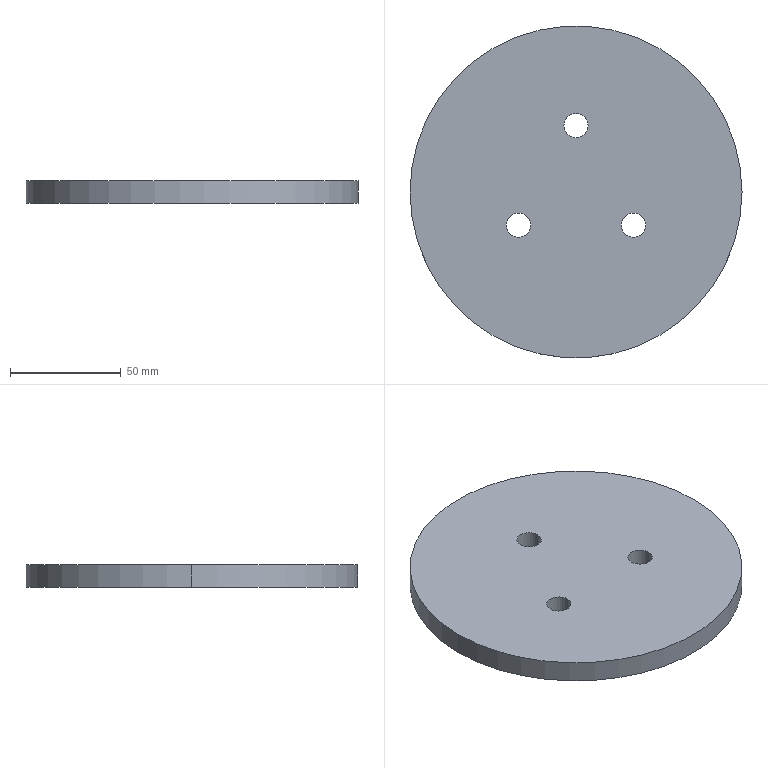Part | SolidWorks | features BaseBody 1 | 1 solid | 10 faces | box 150 x 150 x 10 mm | volume 173864 mm3 | cylinder 8 | plane 2 | commonest cylinder face diameters 11 x6 150 x2
STEP:
#1=CARTESIAN_POINT('',(5.5,30.,-770.));
#2=VERTEX_POINT('',#1);
#3=CARTESIAN_POINT('',(-5.5,30.,-770.));
#4=VERTEX_POINT('',#3);
#5=CARTESIAN_POINT('',(0.,30.,-770.));
#6=DIRECTION('',(0.,0.,-1.));
#7=DIRECTION('',(-1.,0.,0.));
#8=AXIS2_PLACEMENT_3D('',#5,#6,#7);
#9=CIRCLE('',#8,5.5);
#10=EDGE_CURVE('',#2,#4,#9,.T.);
#11=ORIENTED_EDGE('',*,*,#10,.F.);
#12=CARTESIAN_POINT('',(5.5,30.,-780.));
#13=VERTEX_POINT('',#12);
#14=CARTESIAN_POINT('',(5.5,30.,-780.));
#15=DIRECTION('',(0.,0.,-1.));
#16=VECTOR('',#15,1000.);
#17=LINE('',#14,#16);
#18=EDGE_CURVE('',#2,#13,#17,.T.);
#19=ORIENTED_EDGE('',*,*,#18,.T.);
#20=CARTESIAN_POINT('',(-5.5,30.,-780.));
#21=VERTEX_POINT('',#20);
#22=CARTESIAN_POINT('',(0.,30.,-780.));
#23=DIRECTION('',(0.,0.,-1.));
#24=DIRECTION('',(-1.,0.,0.));
#25=AXIS2_PLACEMENT_3D('',#22,#23,#24);
#26=CIRCLE('',#25,5.5);
#27=EDGE_CURVE('',#13,#21,#26,.T.);
#28=ORIENTED_EDGE('',*,*,#27,.T.);
#29=CARTESIAN_POINT('',(-5.5,30.,-780.));
#30=DIRECTION('',(0.,0.,-1.));
#31=VECTOR('',#30,1000.);
#32=LINE('',#29,#31);
#33=EDGE_CURVE('',#4,#21,#32,.T.);
#34=ORIENTED_EDGE('',*,*,#33,.F.);
#35=EDGE_LOOP('',(#11,#19,#28,#34));
#36=FACE_OUTER_BOUND('',#35,.T.);
#37=CARTESIAN_POINT('',(0.,30.,-780.));
#38=DIRECTION('',(0.,0.,-1.));
#39=DIRECTION('',(-1.,0.,0.));
#40=AXIS2_PLACEMENT_3D('',#37,#38,#39);
#41=CYLINDRICAL_SURFACE('',#40,5.5);
#42=ADVANCED_FACE('',(#36),#41,.F.);
#43=CARTESIAN_POINT('',(31.481,-15.,-770.));
#44=VERTEX_POINT('',#43);
#45=CARTESIAN_POINT('',(20.481,-15.,-770.));
#46=VERTEX_POINT('',#45);
#47=CARTESIAN_POINT('',(25.981,-15.,-770.));
#48=DIRECTION('',(0.,0.,-1.));
#49=DIRECTION('',(-1.,0.,0.));
#50=AXIS2_PLACEMENT_3D('',#47,#48,#49);
#51=CIRCLE('',#50,5.5);
#52=EDGE_CURVE('',#44,#46,#51,.T.);
#53=ORIENTED_EDGE('',*,*,#52,.F.);
#54=CARTESIAN_POINT('',(31.481,-15.,-780.));
#55=VERTEX_POINT('',#54);
#56=CARTESIAN_POINT('',(31.481,-15.,-780.));
#57=DIRECTION('',(0.,0.,-1.));
#58=VECTOR('',#57,1000.);
#59=LINE('',#56,#58);
#60=EDGE_CURVE('',#44,#55,#59,.T.);
#61=ORIENTED_EDGE('',*,*,#60,.T.);
#62=CARTESIAN_POINT('',(20.481,-15.,-780.));
#63=VERTEX_POINT('',#62);
#64=CARTESIAN_POINT('',(25.981,-15.,-780.));
#65=DIRECTION('',(0.,0.,-1.));
#66=DIRECTION('',(-1.,0.,0.));
#67=AXIS2_PLACEMENT_3D('',#64,#65,#66);
#68=CIRCLE('',#67,5.5);
#69=EDGE_CURVE('',#55,#63,#68,.T.);
#70=ORIENTED_EDGE('',*,*,#69,.T.);
#71=CARTESIAN_POINT('',(20.481,-15.,-780.));
#72=DIRECTION('',(0.,0.,-1.));
#73=VECTOR('',#72,1000.);
#74=LINE('',#71,#73);
#75=EDGE_CURVE('',#46,#63,#74,.T.);
#76=ORIENTED_EDGE('',*,*,#75,.F.);
#77=EDGE_LOOP('',(#53,#61,#70,#76));
#78=FACE_OUTER_BOUND('',#77,.T.);
#79=CARTESIAN_POINT('',(25.981,-15.,-780.));
#80=DIRECTION('',(0.,0.,-1.));
#81=DIRECTION('',(-1.,0.,0.));
#82=AXIS2_PLACEMENT_3D('',#79,#80,#81);
#83=CYLINDRICAL_SURFACE('',#82,5.5);
#84=ADVANCED_FACE('',(#78),#83,.F.);
#85=CARTESIAN_POINT('',(-20.481,-15.,-770.));
#86=VERTEX_POINT('',#85);
#87=CARTESIAN_POINT('',(-31.481,-15.,-770.));
#88=VERTEX_POINT('',#87);
#89=CARTESIAN_POINT('',(-25.981,-15.,-770.));
#90=DIRECTION('',(0.,0.,-1.));
#91=DIRECTION('',(-1.,0.,0.));
#92=AXIS2_PLACEMENT_3D('',#89,#90,#91);
#93=CIRCLE('',#92,5.5);
#94=EDGE_CURVE('',#86,#88,#93,.T.);
#95=ORIENTED_EDGE('',*,*,#94,.F.);
#96=CARTESIAN_POINT('',(-20.481,-15.,-780.));
#97=VERTEX_POINT('',#96);
#98=CARTESIAN_POINT('',(-20.481,-15.,-780.));
#99=DIRECTION('',(0.,0.,-1.));
#100=VECTOR('',#99,1000.);
#101=LINE('',#98,#100);
#102=EDGE_CURVE('',#86,#97,#101,.T.);
#103=ORIENTED_EDGE('',*,*,#102,.T.);
#104=CARTESIAN_POINT('',(-31.481,-15.,-780.));
#105=VERTEX_POINT('',#104);
#106=CARTESIAN_POINT('',(-25.981,-15.,-780.));
#107=DIRECTION('',(0.,0.,-1.));
#108=DIRECTION('',(-1.,0.,0.));
#109=AXIS2_PLACEMENT_3D('',#106,#107,#108);
#110=CIRCLE('',#109,5.5);
#111=EDGE_CURVE('',#97,#105,#110,.T.);
#112=ORIENTED_EDGE('',*,*,#111,.T.);
#113=CARTESIAN_POINT('',(-31.481,-15.,-780.));
#114=DIRECTION('',(0.,0.,-1.));
#115=VECTOR('',#114,1000.);
#116=LINE('',#113,#115);
#117=EDGE_CURVE('',#88,#105,#116,.T.);
#118=ORIENTED_EDGE('',*,*,#117,.F.);
#119=EDGE_LOOP('',(#95,#103,#112,#118));
#120=FACE_OUTER_BOUND('',#119,.T.);
#121=CARTESIAN_POINT('',(-25.981,-15.,-780.));
#122=DIRECTION('',(0.,0.,-1.));
#123=DIRECTION('',(-1.,0.,0.));
#124=AXIS2_PLACEMENT_3D('',#121,#122,#123);
#125=CYLINDRICAL_SURFACE('',#124,5.5);
#126=ADVANCED_FACE('',(#120),#125,.F.);
#127=CARTESIAN_POINT('',(-75.,0.,-780.));
#128=VERTEX_POINT('',#127);
#129=CARTESIAN_POINT('',(75.,0.,-780.));
#130=VERTEX_POINT('',#129);
#131=CARTESIAN_POINT('',(0.,0.,-780.));
#132=DIRECTION('',(0.,0.,-1.));
#133=DIRECTION('',(-1.,0.,0.));
#134=AXIS2_PLACEMENT_3D('',#131,#132,#133);
#135=CIRCLE('',#134,75.);
#136=EDGE_CURVE('',#128,#130,#135,.T.);
#137=ORIENTED_EDGE('',*,*,#136,.F.);
#138=CARTESIAN_POINT('',(-75.,0.,-770.));
#139=VERTEX_POINT('',#138);
#140=CARTESIAN_POINT('',(-75.,0.,-780.));
#141=DIRECTION('',(0.,0.,1.));
#142=VECTOR('',#141,1000.);
#143=LINE('',#140,#142);
#144=EDGE_CURVE('',#128,#139,#143,.T.);
#145=ORIENTED_EDGE('',*,*,#144,.T.);
#146=CARTESIAN_POINT('',(75.,0.,-770.));
#147=VERTEX_POINT('',#146);
#148=CARTESIAN_POINT('',(0.,0.,-770.));
#149=DIRECTION('',(0.,0.,-1.));
#150=DIRECTION('',(-1.,0.,0.));
#151=AXIS2_PLACEMENT_3D('',#148,#149,#150);
#152=CIRCLE('',#151,75.);
#153=EDGE_CURVE('',#139,#147,#152,.T.);
#154=ORIENTED_EDGE('',*,*,#153,.T.);
#155=CARTESIAN_POINT('',(75.,0.,-780.));
#156=DIRECTION('',(0.,0.,1.));
#157=VECTOR('',#156,1000.);
#158=LINE('',#155,#157);
#159=EDGE_CURVE('',#130,#147,#158,.T.);
#160=ORIENTED_EDGE('',*,*,#159,.F.);
#161=EDGE_LOOP('',(#137,#145,#154,#160));
#162=FACE_OUTER_BOUND('',#161,.T.);
#163=CARTESIAN_POINT('',(0.,0.,-780.));
#164=DIRECTION('',(0.,0.,1.));
#165=DIRECTION('',(1.,0.,0.));
#166=AXIS2_PLACEMENT_3D('',#163,#164,#165);
#167=CYLINDRICAL_SURFACE('',#166,75.);
#168=ADVANCED_FACE('',(#162),#167,.T.);
#169=ORIENTED_EDGE('',*,*,#144,.F.);
#170=CARTESIAN_POINT('',(0.,0.,-780.));
#171=DIRECTION('',(0.,0.,-1.));
#172=DIRECTION('',(-1.,0.,0.));
#173=AXIS2_PLACEMENT_3D('',#170,#171,#172);
#174=CIRCLE('',#173,75.);
#175=EDGE_CURVE('',#130,#128,#174,.T.);
#176=ORIENTED_EDGE('',*,*,#175,.F.);
#177=ORIENTED_EDGE('',*,*,#159,.T.);
#178=CARTESIAN_POINT('',(0.,0.,-770.));
#179=DIRECTION('',(0.,0.,-1.));
#180=DIRECTION('',(-1.,0.,0.));
#181=AXIS2_PLACEMENT_3D('',#178,#179,#180);
#182=CIRCLE('',#181,75.);
#183=EDGE_CURVE('',#147,#139,#182,.T.);
#184=ORIENTED_EDGE('',*,*,#183,.T.);
#185=EDGE_LOOP('',(#169,#176,#177,#184));
#186=FACE_OUTER_BOUND('',#185,.T.);
#187=CARTESIAN_POINT('',(0.,0.,-780.));
#188=DIRECTION('',(0.,0.,1.));
#189=DIRECTION('',(1.,0.,0.));
#190=AXIS2_PLACEMENT_3D('',#187,#188,#189);
#191=CYLINDRICAL_SURFACE('',#190,75.);
#192=ADVANCED_FACE('',(#186),#191,.T.);
#193=CARTESIAN_POINT('',(0.,30.,-780.));
#194=DIRECTION('',(0.,0.,-1.));
#195=DIRECTION('',(-1.,0.,0.));
#196=AXIS2_PLACEMENT_3D('',#193,#194,#195);
#197=CIRCLE('',#196,5.5);
#198=EDGE_CURVE('',#21,#13,#197,.T.);
#199=ORIENTED_EDGE('',*,*,#198,.F.);
#200=ORIENTED_EDGE('',*,*,#27,.F.);
#201=EDGE_LOOP('',(#199,#200));
#202=FACE_BOUND('',#201,.T.);
#203=CARTESIAN_POINT('',(25.981,-15.,-780.));
#204=DIRECTION('',(0.,0.,-1.));
#205=DIRECTION('',(-1.,0.,0.));
#206=AXIS2_PLACEMENT_3D('',#203,#204,#205);
#207=CIRCLE('',#206,5.5);
#208=EDGE_CURVE('',#63,#55,#207,.T.);
#209=ORIENTED_EDGE('',*,*,#208,.F.);
#210=ORIENTED_EDGE('',*,*,#69,.F.);
#211=EDGE_LOOP('',(#209,#210));
#212=FACE_BOUND('',#211,.T.);
#213=CARTESIAN_POINT('',(-25.981,-15.,-780.));
#214=DIRECTION('',(0.,0.,-1.));
#215=DIRECTION('',(-1.,0.,0.));
#216=AXIS2_PLACEMENT_3D('',#213,#214,#215);
#217=CIRCLE('',#216,5.5);
#218=EDGE_CURVE('',#105,#97,#217,.T.);
#219=ORIENTED_EDGE('',*,*,#218,.F.);
#220=ORIENTED_EDGE('',*,*,#111,.F.);
#221=EDGE_LOOP('',(#219,#220));
#222=FACE_BOUND('',#221,.T.);
#223=ORIENTED_EDGE('',*,*,#175,.T.);
#224=ORIENTED_EDGE('',*,*,#136,.T.);
#225=EDGE_LOOP('',(#223,#224));
#226=FACE_OUTER_BOUND('',#225,.T.);
#227=CARTESIAN_POINT('',(0.,0.,-780.));
#228=DIRECTION('',(0.,0.,-1.));
#229=DIRECTION('',(-1.,0.,0.));
#230=AXIS2_PLACEMENT_3D('',#227,#228,#229);
#231=PLANE('',#230);
#232=ADVANCED_FACE('',(#202,#212,#222,#226),#231,.T.);
#233=CARTESIAN_POINT('',(0.,30.,-770.));
#234=DIRECTION('',(0.,0.,-1.));
#235=DIRECTION('',(-1.,0.,0.));
#236=AXIS2_PLACEMENT_3D('',#233,#234,#235);
#237=CIRCLE('',#236,5.5);
#238=EDGE_CURVE('',#4,#2,#237,.T.);
#239=ORIENTED_EDGE('',*,*,#238,.T.);
#240=ORIENTED_EDGE('',*,*,#10,.T.);
#241=EDGE_LOOP('',(#239,#240));
#242=FACE_BOUND('',#241,.T.);
#243=CARTESIAN_POINT('',(25.981,-15.,-770.));
#244=DIRECTION('',(0.,0.,-1.));
#245=DIRECTION('',(-1.,0.,0.));
#246=AXIS2_PLACEMENT_3D('',#243,#244,#245);
#247=CIRCLE('',#246,5.5);
#248=EDGE_CURVE('',#46,#44,#247,.T.);
#249=ORIENTED_EDGE('',*,*,#248,.T.);
#250=ORIENTED_EDGE('',*,*,#52,.T.);
#251=EDGE_LOOP('',(#249,#250));
#252=FACE_BOUND('',#251,.T.);
#253=CARTESIAN_POINT('',(-25.981,-15.,-770.));
#254=DIRECTION('',(0.,0.,-1.));
#255=DIRECTION('',(-1.,0.,0.));
#256=AXIS2_PLACEMENT_3D('',#253,#254,#255);
#257=CIRCLE('',#256,5.5);
#258=EDGE_CURVE('',#88,#86,#257,.T.);
#259=ORIENTED_EDGE('',*,*,#258,.T.);
#260=ORIENTED_EDGE('',*,*,#94,.T.);
#261=EDGE_LOOP('',(#259,#260));
#262=FACE_BOUND('',#261,.T.);
#263=ORIENTED_EDGE('',*,*,#183,.F.);
#264=ORIENTED_EDGE('',*,*,#153,.F.);
#265=EDGE_LOOP('',(#263,#264));
#266=FACE_OUTER_BOUND('',#265,.T.);
#267=CARTESIAN_POINT('',(0.,0.,-770.));
#268=DIRECTION('',(0.,0.,-1.));
#269=DIRECTION('',(-1.,0.,0.));
#270=AXIS2_PLACEMENT_3D('',#267,#268,#269);
#271=PLANE('',#270);
#272=ADVANCED_FACE('',(#242,#252,#262,#266),#271,.F.);
#273=ORIENTED_EDGE('',*,*,#102,.F.);
#274=ORIENTED_EDGE('',*,*,#258,.F.);
#275=ORIENTED_EDGE('',*,*,#117,.T.);
#276=ORIENTED_EDGE('',*,*,#218,.T.);
#277=EDGE_LOOP('',(#273,#274,#275,#276));
#278=FACE_OUTER_BOUND('',#277,.T.);
#279=CARTESIAN_POINT('',(-25.981,-15.,-780.));
#280=DIRECTION('',(0.,0.,-1.));
#281=DIRECTION('',(-1.,0.,0.));
#282=AXIS2_PLACEMENT_3D('',#279,#280,#281);
#283=CYLINDRICAL_SURFACE('',#282,5.5);
#284=ADVANCED_FACE('',(#278),#283,.F.);
#285=ORIENTED_EDGE('',*,*,#60,.F.);
#286=ORIENTED_EDGE('',*,*,#248,.F.);
#287=ORIENTED_EDGE('',*,*,#75,.T.);
#288=ORIENTED_EDGE('',*,*,#208,.T.);
#289=EDGE_LOOP('',(#285,#286,#287,#288));
#290=FACE_OUTER_BOUND('',#289,.T.);
#291=CARTESIAN_POINT('',(25.981,-15.,-780.));
#292=DIRECTION('',(0.,0.,-1.));
#293=DIRECTION('',(-1.,0.,0.));
#294=AXIS2_PLACEMENT_3D('',#291,#292,#293);
#295=CYLINDRICAL_SURFACE('',#294,5.5);
#296=ADVANCED_FACE('',(#290),#295,.F.);
#297=ORIENTED_EDGE('',*,*,#18,.F.);
#298=ORIENTED_EDGE('',*,*,#238,.F.);
#299=ORIENTED_EDGE('',*,*,#33,.T.);
#300=ORIENTED_EDGE('',*,*,#198,.T.);
#301=EDGE_LOOP('',(#297,#298,#299,#300));
#302=FACE_OUTER_BOUND('',#301,.T.);
#303=CARTESIAN_POINT('',(0.,30.,-780.));
#304=DIRECTION('',(0.,0.,-1.));
#305=DIRECTION('',(-1.,0.,0.));
#306=AXIS2_PLACEMENT_3D('',#303,#304,#305);
#307=CYLINDRICAL_SURFACE('',#306,5.5);
#308=ADVANCED_FACE('',(#302),#307,.F.);
#309=CLOSED_SHELL('',(#42,#84,#126,#168,#192,#232,#272,#284,#296,#308));
#310=MANIFOLD_SOLID_BREP('',#309);
#311=CARTESIAN_POINT('',(0.,0.,0.));
#312=DIRECTION('',(0.,0.,1.));
#313=DIRECTION('',(1.,0.,0.));
#314=AXIS2_PLACEMENT_3D('',#311,#312,#313);
#315=(LENGTH_UNIT()NAMED_UNIT(*)SI_UNIT(.MILLI.,.METRE.));
#316=UNCERTAINTY_MEASURE_WITH_UNIT(LENGTH_MEASURE(0.00001),#315,'','');
#317=(NAMED_UNIT(*)PLANE_ANGLE_UNIT()SI_UNIT($,.RADIAN.));
#318=(NAMED_UNIT(*)SI_UNIT($,.STERADIAN.)SOLID_ANGLE_UNIT());
#319=(GEOMETRIC_REPRESENTATION_CONTEXT(3)GLOBAL_UNCERTAINTY_ASSIGNED_CONTEXT((#316))GLOBAL_UNIT_ASSIGNED_CONTEXT((#315,#317,#318))REPRESENTATION_CONTEXT('',''));
#320=ADVANCED_BREP_SHAPE_REPRESENTATION('',(#310,#314),#319);